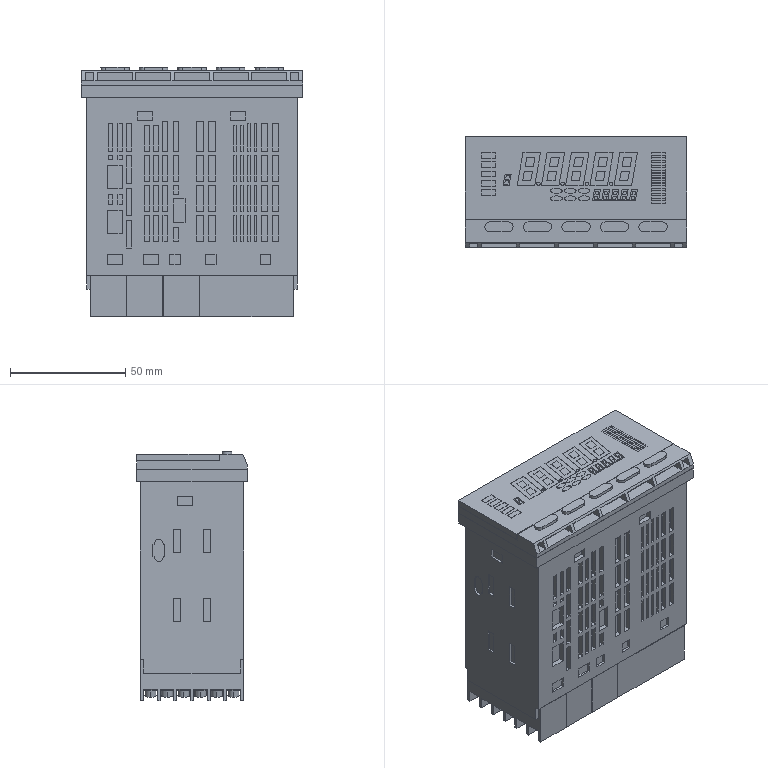Part | STEP file | K3HB_V_BASE | 1 solid | 1805 faces | box 96 x 48 x 108.3 mm | volume 416393 mm3 | plane 1603 | cylinder 190 | spline 12 | commonest cylinder face diameters 5 x52 1.256 x26 2.056 x26 1.959 x25 2.759 x25 4.195 x15